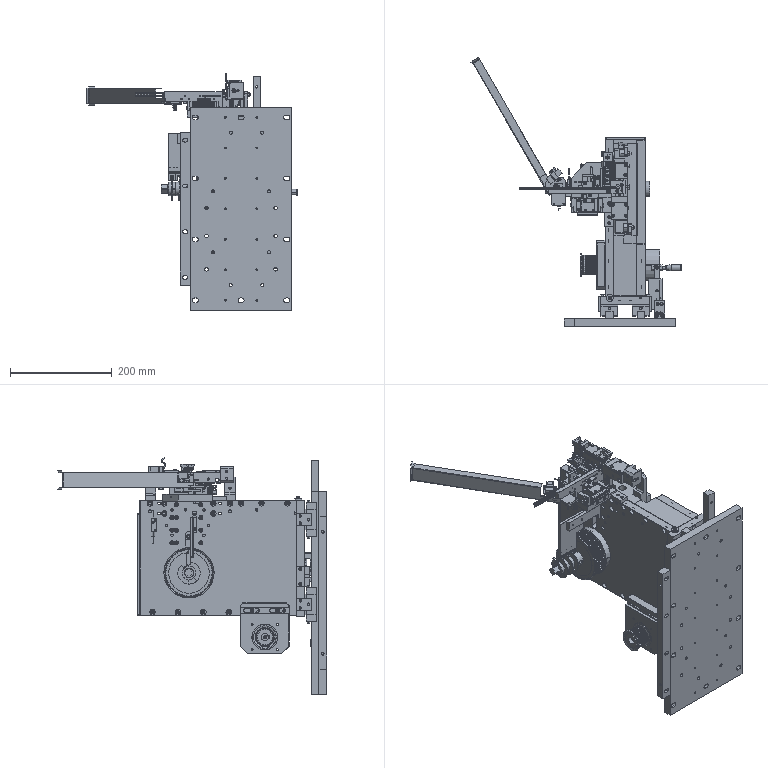Part | NX | 197 solids | 17824 faces | volume 6383944 mm3 | plane 8524 | cylinder 6166 | torus 1403 | cone 1287 | sphere 315 | spline 129 | commonest cylinder face diameters 0.2 x628 5 x553 0.8 x359 0.4 x286 0.6 x277 3.3 x266